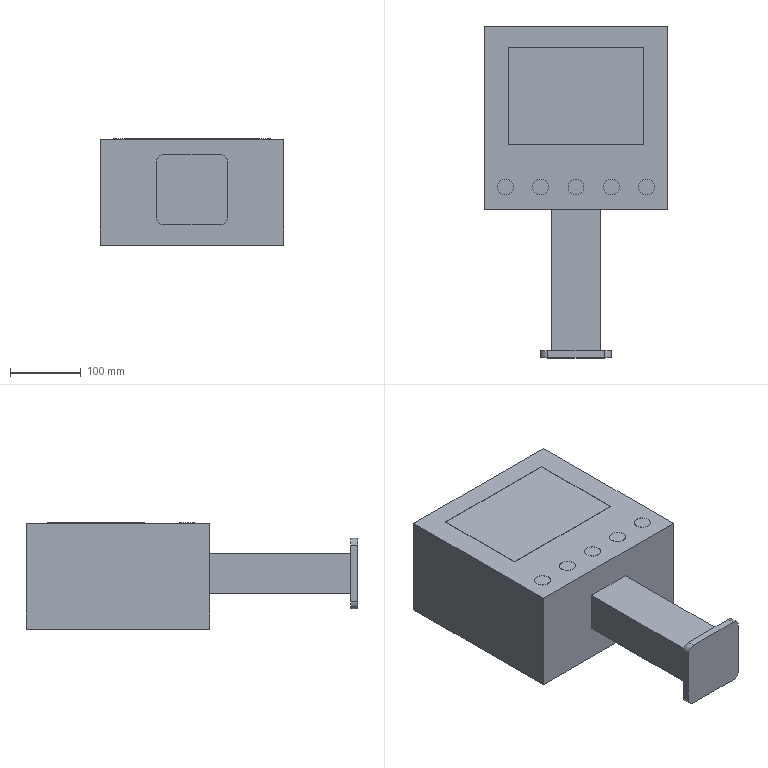Part | SolidWorks | features ICE 3, Extrusion 1, Fillet 1 | 1 solid | 40 faces | box 260 x 470 x 150.5 mm | volume 11032431 mm3 | plane 26 | cylinder 14 | commonest cylinder face diameters 22.5 x10 20 x4
STEP:
#1=CARTESIAN_POINT('',(11.25,-98.,150.5));
#2=VERTEX_POINT('',#1);
#3=CARTESIAN_POINT('',(-11.25,-98.,150.5));
#4=VERTEX_POINT('',#3);
#5=CARTESIAN_POINT('',(0.,-98.,150.5));
#6=DIRECTION('',(0.,0.,1.));
#7=DIRECTION('',(-1.,0.,0.));
#8=AXIS2_PLACEMENT_3D('',#5,#6,#7);
#9=CIRCLE('',#8,11.25);
#10=EDGE_CURVE('',#2,#4,#9,.T.);
#11=ORIENTED_EDGE('',*,*,#10,.F.);
#12=CARTESIAN_POINT('',(11.25,-98.,150.));
#13=VERTEX_POINT('',#12);
#14=CARTESIAN_POINT('',(11.25,-98.,150.5));
#15=DIRECTION('',(0.,0.,-1.));
#16=VECTOR('',#15,1000.);
#17=LINE('',#14,#16);
#18=EDGE_CURVE('',#2,#13,#17,.T.);
#19=ORIENTED_EDGE('',*,*,#18,.T.);
#20=CARTESIAN_POINT('',(-11.25,-98.,150.));
#21=VERTEX_POINT('',#20);
#22=CARTESIAN_POINT('',(0.,-98.,150.));
#23=DIRECTION('',(0.,0.,1.));
#24=DIRECTION('',(-1.,0.,0.));
#25=AXIS2_PLACEMENT_3D('',#22,#23,#24);
#26=CIRCLE('',#25,11.25);
#27=EDGE_CURVE('',#13,#21,#26,.T.);
#28=ORIENTED_EDGE('',*,*,#27,.T.);
#29=CARTESIAN_POINT('',(-11.25,-98.,150.5));
#30=DIRECTION('',(0.,0.,-1.));
#31=VECTOR('',#30,1000.);
#32=LINE('',#29,#31);
#33=EDGE_CURVE('',#4,#21,#32,.T.);
#34=ORIENTED_EDGE('',*,*,#33,.F.);
#35=EDGE_LOOP('',(#11,#19,#28,#34));
#36=FACE_OUTER_BOUND('',#35,.T.);
#37=CARTESIAN_POINT('',(0.,-98.,150.5));
#38=DIRECTION('',(0.,0.,-1.));
#39=DIRECTION('',(-1.,0.,0.));
#40=AXIS2_PLACEMENT_3D('',#37,#38,#39);
#41=CYLINDRICAL_SURFACE('',#40,11.25);
#42=ADVANCED_FACE('',(#36),#41,.T.);
#43=CARTESIAN_POINT('',(111.25,-98.,150.5));
#44=VERTEX_POINT('',#43);
#45=CARTESIAN_POINT('',(88.75,-98.,150.5));
#46=VERTEX_POINT('',#45);
#47=CARTESIAN_POINT('',(100.,-98.,150.5));
#48=DIRECTION('',(0.,0.,1.));
#49=DIRECTION('',(-1.,0.,0.));
#50=AXIS2_PLACEMENT_3D('',#47,#48,#49);
#51=CIRCLE('',#50,11.25);
#52=EDGE_CURVE('',#44,#46,#51,.T.);
#53=ORIENTED_EDGE('',*,*,#52,.F.);
#54=CARTESIAN_POINT('',(111.25,-98.,150.));
#55=VERTEX_POINT('',#54);
#56=CARTESIAN_POINT('',(111.25,-98.,150.5));
#57=DIRECTION('',(0.,0.,-1.));
#58=VECTOR('',#57,1000.);
#59=LINE('',#56,#58);
#60=EDGE_CURVE('',#44,#55,#59,.T.);
#61=ORIENTED_EDGE('',*,*,#60,.T.);
#62=CARTESIAN_POINT('',(88.75,-98.,150.));
#63=VERTEX_POINT('',#62);
#64=CARTESIAN_POINT('',(100.,-98.,150.));
#65=DIRECTION('',(0.,0.,1.));
#66=DIRECTION('',(-1.,0.,0.));
#67=AXIS2_PLACEMENT_3D('',#64,#65,#66);
#68=CIRCLE('',#67,11.25);
#69=EDGE_CURVE('',#55,#63,#68,.T.);
#70=ORIENTED_EDGE('',*,*,#69,.T.);
#71=CARTESIAN_POINT('',(88.75,-98.,150.5));
#72=DIRECTION('',(0.,0.,-1.));
#73=VECTOR('',#72,1000.);
#74=LINE('',#71,#73);
#75=EDGE_CURVE('',#46,#63,#74,.T.);
#76=ORIENTED_EDGE('',*,*,#75,.F.);
#77=EDGE_LOOP('',(#53,#61,#70,#76));
#78=FACE_OUTER_BOUND('',#77,.T.);
#79=CARTESIAN_POINT('',(100.,-98.,150.5));
#80=DIRECTION('',(0.,0.,-1.));
#81=DIRECTION('',(-1.,0.,0.));
#82=AXIS2_PLACEMENT_3D('',#79,#80,#81);
#83=CYLINDRICAL_SURFACE('',#82,11.25);
#84=ADVANCED_FACE('',(#78),#83,.T.);
#85=CARTESIAN_POINT('',(61.25,-98.,150.5));
#86=VERTEX_POINT('',#85);
#87=CARTESIAN_POINT('',(38.75,-98.,150.5));
#88=VERTEX_POINT('',#87);
#89=CARTESIAN_POINT('',(50.,-98.,150.5));
#90=DIRECTION('',(0.,0.,1.));
#91=DIRECTION('',(-1.,0.,0.));
#92=AXIS2_PLACEMENT_3D('',#89,#90,#91);
#93=CIRCLE('',#92,11.25);
#94=EDGE_CURVE('',#86,#88,#93,.T.);
#95=ORIENTED_EDGE('',*,*,#94,.F.);
#96=CARTESIAN_POINT('',(61.25,-98.,150.));
#97=VERTEX_POINT('',#96);
#98=CARTESIAN_POINT('',(61.25,-98.,150.5));
#99=DIRECTION('',(0.,0.,-1.));
#100=VECTOR('',#99,1000.);
#101=LINE('',#98,#100);
#102=EDGE_CURVE('',#86,#97,#101,.T.);
#103=ORIENTED_EDGE('',*,*,#102,.T.);
#104=CARTESIAN_POINT('',(38.75,-98.,150.));
#105=VERTEX_POINT('',#104);
#106=CARTESIAN_POINT('',(50.,-98.,150.));
#107=DIRECTION('',(0.,0.,1.));
#108=DIRECTION('',(-1.,0.,0.));
#109=AXIS2_PLACEMENT_3D('',#106,#107,#108);
#110=CIRCLE('',#109,11.25);
#111=EDGE_CURVE('',#97,#105,#110,.T.);
#112=ORIENTED_EDGE('',*,*,#111,.T.);
#113=CARTESIAN_POINT('',(38.75,-98.,150.5));
#114=DIRECTION('',(0.,0.,-1.));
#115=VECTOR('',#114,1000.);
#116=LINE('',#113,#115);
#117=EDGE_CURVE('',#88,#105,#116,.T.);
#118=ORIENTED_EDGE('',*,*,#117,.F.);
#119=EDGE_LOOP('',(#95,#103,#112,#118));
#120=FACE_OUTER_BOUND('',#119,.T.);
#121=CARTESIAN_POINT('',(50.,-98.,150.5));
#122=DIRECTION('',(0.,0.,-1.));
#123=DIRECTION('',(-1.,0.,0.));
#124=AXIS2_PLACEMENT_3D('',#121,#122,#123);
#125=CYLINDRICAL_SURFACE('',#124,11.25);
#126=ADVANCED_FACE('',(#120),#125,.T.);
#127=CARTESIAN_POINT('',(-38.75,-98.,150.5));
#128=VERTEX_POINT('',#127);
#129=CARTESIAN_POINT('',(-61.25,-98.,150.5));
#130=VERTEX_POINT('',#129);
#131=CARTESIAN_POINT('',(-50.,-98.,150.5));
#132=DIRECTION('',(0.,0.,1.));
#133=DIRECTION('',(1.,0.,0.));
#134=AXIS2_PLACEMENT_3D('',#131,#132,#133);
#135=CIRCLE('',#134,11.25);
#136=EDGE_CURVE('',#128,#130,#135,.T.);
#137=ORIENTED_EDGE('',*,*,#136,.F.);
#138=CARTESIAN_POINT('',(-38.75,-98.,150.));
#139=VERTEX_POINT('',#138);
#140=CARTESIAN_POINT('',(-38.75,-98.,150.5));
#141=DIRECTION('',(0.,0.,-1.));
#142=VECTOR('',#141,1000.);
#143=LINE('',#140,#142);
#144=EDGE_CURVE('',#128,#139,#143,.T.);
#145=ORIENTED_EDGE('',*,*,#144,.T.);
#146=CARTESIAN_POINT('',(-61.25,-98.,150.));
#147=VERTEX_POINT('',#146);
#148=CARTESIAN_POINT('',(-50.,-98.,150.));
#149=DIRECTION('',(0.,0.,1.));
#150=DIRECTION('',(1.,0.,0.));
#151=AXIS2_PLACEMENT_3D('',#148,#149,#150);
#152=CIRCLE('',#151,11.25);
#153=EDGE_CURVE('',#139,#147,#152,.T.);
#154=ORIENTED_EDGE('',*,*,#153,.T.);
#155=CARTESIAN_POINT('',(-61.25,-98.,150.5));
#156=DIRECTION('',(0.,0.,-1.));
#157=VECTOR('',#156,1000.);
#158=LINE('',#155,#157);
#159=EDGE_CURVE('',#130,#147,#158,.T.);
#160=ORIENTED_EDGE('',*,*,#159,.F.);
#161=EDGE_LOOP('',(#137,#145,#154,#160));
#162=FACE_OUTER_BOUND('',#161,.T.);
#163=CARTESIAN_POINT('',(-50.,-98.,150.5));
#164=DIRECTION('',(0.,0.,-1.));
#165=DIRECTION('',(-1.,0.,0.));
#166=AXIS2_PLACEMENT_3D('',#163,#164,#165);
#167=CYLINDRICAL_SURFACE('',#166,11.25);
#168=ADVANCED_FACE('',(#162),#167,.T.);
#169=CARTESIAN_POINT('',(-88.75,-98.,150.5));
#170=VERTEX_POINT('',#169);
#171=CARTESIAN_POINT('',(-111.25,-98.,150.5));
#172=VERTEX_POINT('',#171);
#173=CARTESIAN_POINT('',(-100.,-98.,150.5));
#174=DIRECTION('',(0.,0.,1.));
#175=DIRECTION('',(1.,0.,0.));
#176=AXIS2_PLACEMENT_3D('',#173,#174,#175);
#177=CIRCLE('',#176,11.25);
#178=EDGE_CURVE('',#170,#172,#177,.T.);
#179=ORIENTED_EDGE('',*,*,#178,.F.);
#180=CARTESIAN_POINT('',(-88.75,-98.,150.));
#181=VERTEX_POINT('',#180);
#182=CARTESIAN_POINT('',(-88.75,-98.,150.5));
#183=DIRECTION('',(0.,0.,-1.));
#184=VECTOR('',#183,1000.);
#185=LINE('',#182,#184);
#186=EDGE_CURVE('',#170,#181,#185,.T.);
#187=ORIENTED_EDGE('',*,*,#186,.T.);
#188=CARTESIAN_POINT('',(-111.25,-98.,150.));
#189=VERTEX_POINT('',#188);
#190=CARTESIAN_POINT('',(-100.,-98.,150.));
#191=DIRECTION('',(0.,0.,1.));
#192=DIRECTION('',(1.,0.,0.));
#193=AXIS2_PLACEMENT_3D('',#190,#191,#192);
#194=CIRCLE('',#193,11.25);
#195=EDGE_CURVE('',#181,#189,#194,.T.);
#196=ORIENTED_EDGE('',*,*,#195,.T.);
#197=CARTESIAN_POINT('',(-111.25,-98.,150.5));
#198=DIRECTION('',(0.,0.,-1.));
#199=VECTOR('',#198,1000.);
#200=LINE('',#197,#199);
#201=EDGE_CURVE('',#172,#189,#200,.T.);
#202=ORIENTED_EDGE('',*,*,#201,.F.);
#203=EDGE_LOOP('',(#179,#187,#196,#202));
#204=FACE_OUTER_BOUND('',#203,.T.);
#205=CARTESIAN_POINT('',(-100.,-98.,150.5));
#206=DIRECTION('',(0.,0.,-1.));
#207=DIRECTION('',(-1.,0.,0.));
#208=AXIS2_PLACEMENT_3D('',#205,#206,#207);
#209=CYLINDRICAL_SURFACE('',#208,11.25);
#210=ADVANCED_FACE('',(#204),#209,.T.);
#211=CARTESIAN_POINT('',(-130.,-130.,0.));
#212=VERTEX_POINT('',#211);
#213=CARTESIAN_POINT('',(130.,-130.,0.));
#214=VERTEX_POINT('',#213);
#215=CARTESIAN_POINT('',(-130.,-130.,0.));
#216=DIRECTION('',(1.,0.,0.));
#217=VECTOR('',#216,1000.);
#218=LINE('',#215,#217);
#219=EDGE_CURVE('',#212,#214,#218,.T.);
#220=ORIENTED_EDGE('',*,*,#219,.T.);
#221=CARTESIAN_POINT('',(130.,-130.,150.));
#222=VERTEX_POINT('',#221);
#223=CARTESIAN_POINT('',(130.,-130.,150.));
#224=DIRECTION('',(0.,0.,-1.));
#225=VECTOR('',#224,1000.);
#226=LINE('',#223,#225);
#227=EDGE_CURVE('',#222,#214,#226,.T.);
#228=ORIENTED_EDGE('',*,*,#227,.F.);
#229=CARTESIAN_POINT('',(-130.,-130.,150.));
#230=VERTEX_POINT('',#229);
#231=CARTESIAN_POINT('',(-130.,-130.,150.));
#232=DIRECTION('',(1.,0.,0.));
#233=VECTOR('',#232,1000.);
#234=LINE('',#231,#233);
#235=EDGE_CURVE('',#230,#222,#234,.T.);
#236=ORIENTED_EDGE('',*,*,#235,.F.);
#237=CARTESIAN_POINT('',(-130.,-130.,150.));
#238=DIRECTION('',(0.,0.,-1.));
#239=VECTOR('',#238,1000.);
#240=LINE('',#237,#239);
#241=EDGE_CURVE('',#230,#212,#240,.T.);
#242=ORIENTED_EDGE('',*,*,#241,.T.);
#243=EDGE_LOOP('',(#220,#228,#236,#242));
#244=FACE_OUTER_BOUND('',#243,.T.);
#245=CARTESIAN_POINT('',(34.037,-130.,49.969));
#246=VERTEX_POINT('',#245);
#247=CARTESIAN_POINT('',(34.037,-130.,107.19));
#248=VERTEX_POINT('',#247);
#249=CARTESIAN_POINT('',(34.037,-130.,107.19));
#250=DIRECTION('',(0.,0.,1.));
#251=VECTOR('',#250,1000.);
#252=LINE('',#249,#251);
#253=EDGE_CURVE('',#246,#248,#252,.T.);
#254=ORIENTED_EDGE('',*,*,#253,.F.);
#255=CARTESIAN_POINT('',(-34.037,-130.,49.969));
#256=VERTEX_POINT('',#255);
#257=CARTESIAN_POINT('',(-34.037,-130.,49.969));
#258=DIRECTION('',(1.,0.,0.));
#259=VECTOR('',#258,1000.);
#260=LINE('',#257,#259);
#261=EDGE_CURVE('',#256,#246,#260,.T.);
#262=ORIENTED_EDGE('',*,*,#261,.F.);
#263=CARTESIAN_POINT('',(-34.037,-130.,107.19));
#264=VERTEX_POINT('',#263);
#265=CARTESIAN_POINT('',(-34.037,-130.,107.19));
#266=DIRECTION('',(0.,0.,-1.));
#267=VECTOR('',#266,1000.);
#268=LINE('',#265,#267);
#269=EDGE_CURVE('',#264,#256,#268,.T.);
#270=ORIENTED_EDGE('',*,*,#269,.F.);
#271=CARTESIAN_POINT('',(-34.037,-130.,107.19));
#272=DIRECTION('',(-1.,0.,0.));
#273=VECTOR('',#272,1000.);
#274=LINE('',#271,#273);
#275=EDGE_CURVE('',#248,#264,#274,.T.);
#276=ORIENTED_EDGE('',*,*,#275,.F.);
#277=EDGE_LOOP('',(#254,#262,#270,#276));
#278=FACE_BOUND('',#277,.T.);
#279=CARTESIAN_POINT('',(-130.,-130.,150.));
#280=DIRECTION('',(0.,1.,0.));
#281=DIRECTION('',(0.,0.,1.));
#282=AXIS2_PLACEMENT_3D('',#279,#280,#281);
#283=PLANE('',#282);
#284=ADVANCED_FACE('',(#244,#278),#283,.F.);
#285=CARTESIAN_POINT('',(130.,130.,0.));
#286=VERTEX_POINT('',#285);
#287=CARTESIAN_POINT('',(130.,130.,0.));
#288=DIRECTION('',(0.,1.,0.));
#289=VECTOR('',#288,1000.);
#290=LINE('',#287,#289);
#291=EDGE_CURVE('',#214,#286,#290,.T.);
#292=ORIENTED_EDGE('',*,*,#291,.T.);
#293=CARTESIAN_POINT('',(130.,130.,150.));
#294=VERTEX_POINT('',#293);
#295=CARTESIAN_POINT('',(130.,130.,150.));
#296=DIRECTION('',(0.,0.,-1.));
#297=VECTOR('',#296,1000.);
#298=LINE('',#295,#297);
#299=EDGE_CURVE('',#294,#286,#298,.T.);
#300=ORIENTED_EDGE('',*,*,#299,.F.);
#301=CARTESIAN_POINT('',(130.,130.,150.));
#302=DIRECTION('',(0.,1.,0.));
#303=VECTOR('',#302,1000.);
#304=LINE('',#301,#303);
#305=EDGE_CURVE('',#222,#294,#304,.T.);
#306=ORIENTED_EDGE('',*,*,#305,.F.);
#307=ORIENTED_EDGE('',*,*,#227,.T.);
#308=EDGE_LOOP('',(#292,#300,#306,#307));
#309=FACE_OUTER_BOUND('',#308,.T.);
#310=CARTESIAN_POINT('',(130.,130.,150.));
#311=DIRECTION('',(-1.,0.,0.));
#312=DIRECTION('',(0.,-1.,0.));
#313=AXIS2_PLACEMENT_3D('',#310,#311,#312);
#314=PLANE('',#313);
#315=ADVANCED_FACE('',(#309),#314,.F.);
#316=CARTESIAN_POINT('',(-130.,130.,0.));
#317=VERTEX_POINT('',#316);
#318=CARTESIAN_POINT('',(-130.,130.,0.));
#319=DIRECTION('',(-1.,0.,0.));
#320=VECTOR('',#319,1000.);
#321=LINE('',#318,#320);
#322=EDGE_CURVE('',#286,#317,#321,.T.);
#323=ORIENTED_EDGE('',*,*,#322,.T.);
#324=CARTESIAN_POINT('',(-130.,130.,150.));
#325=VERTEX_POINT('',#324);
#326=CARTESIAN_POINT('',(-130.,130.,150.));
#327=DIRECTION('',(0.,0.,-1.));
#328=VECTOR('',#327,1000.);
#329=LINE('',#326,#328);
#330=EDGE_CURVE('',#325,#317,#329,.T.);
#331=ORIENTED_EDGE('',*,*,#330,.F.);
#332=CARTESIAN_POINT('',(-130.,130.,150.));
#333=DIRECTION('',(-1.,0.,0.));
#334=VECTOR('',#333,1000.);
#335=LINE('',#332,#334);
#336=EDGE_CURVE('',#294,#325,#335,.T.);
#337=ORIENTED_EDGE('',*,*,#336,.F.);
#338=ORIENTED_EDGE('',*,*,#299,.T.);
#339=EDGE_LOOP('',(#323,#331,#337,#338));
#340=FACE_OUTER_BOUND('',#339,.T.);
#341=CARTESIAN_POINT('',(-130.,130.,150.));
#342=DIRECTION('',(0.,-1.,0.));
#343=DIRECTION('',(0.,0.,-1.));
#344=AXIS2_PLACEMENT_3D('',#341,#342,#343);
#345=PLANE('',#344);
#346=ADVANCED_FACE('',(#340),#345,.F.);
#347=CARTESIAN_POINT('',(-130.,130.,0.));
#348=DIRECTION('',(0.,-1.,0.));
#349=VECTOR('',#348,1000.);
#350=LINE('',#347,#349);
#351=EDGE_CURVE('',#317,#212,#350,.T.);
#352=ORIENTED_EDGE('',*,*,#351,.T.);
#353=ORIENTED_EDGE('',*,*,#241,.F.);
#354=CARTESIAN_POINT('',(-130.,130.,150.));
#355=DIRECTION('',(0.,-1.,0.));
#356=VECTOR('',#355,1000.);
#357=LINE('',#354,#356);
#358=EDGE_CURVE('',#325,#230,#357,.T.);
#359=ORIENTED_EDGE('',*,*,#358,.F.);
#360=ORIENTED_EDGE('',*,*,#330,.T.);
#361=EDGE_LOOP('',(#352,#353,#359,#360));
#362=FACE_OUTER_BOUND('',#361,.T.);
#363=CARTESIAN_POINT('',(-130.,130.,150.));
#364=DIRECTION('',(1.,0.,0.));
#365=DIRECTION('',(0.,0.,-1.));
#366=AXIS2_PLACEMENT_3D('',#363,#364,#365);
#367=PLANE('',#366);
#368=ADVANCED_FACE('',(#362),#367,.F.);
#369=CARTESIAN_POINT('',(0.,-98.,150.));
#370=DIRECTION('',(0.,0.,1.));
#371=DIRECTION('',(-1.,0.,0.));
#372=AXIS2_PLACEMENT_3D('',#369,#370,#371);
#373=CIRCLE('',#372,11.25);
#374=EDGE_CURVE('',#21,#13,#373,.T.);
#375=ORIENTED_EDGE('',*,*,#374,.F.);
#376=ORIENTED_EDGE('',*,*,#27,.F.);
#377=EDGE_LOOP('',(#375,#376));
#378=FACE_BOUND('',#377,.T.);
#379=CARTESIAN_POINT('',(100.,-98.,150.));
#380=DIRECTION('',(0.,0.,1.));
#381=DIRECTION('',(-1.,0.,0.));
#382=AXIS2_PLACEMENT_3D('',#379,#380,#381);
#383=CIRCLE('',#382,11.25);
#384=EDGE_CURVE('',#63,#55,#383,.T.);
#385=ORIENTED_EDGE('',*,*,#384,.F.);
#386=ORIENTED_EDGE('',*,*,#69,.F.);
#387=EDGE_LOOP('',(#385,#386));
#388=FACE_BOUND('',#387,.T.);
#389=CARTESIAN_POINT('',(50.,-98.,150.));
#390=DIRECTION('',(0.,0.,1.));
#391=DIRECTION('',(-1.,0.,0.));
#392=AXIS2_PLACEMENT_3D('',#389,#390,#391);
#393=CIRCLE('',#392,11.25);
#394=EDGE_CURVE('',#105,#97,#393,.T.);
#395=ORIENTED_EDGE('',*,*,#394,.F.);
#396=ORIENTED_EDGE('',*,*,#111,.F.);
#397=EDGE_LOOP('',(#395,#396));
#398=FACE_BOUND('',#397,.T.);
#399=CARTESIAN_POINT('',(-50.,-98.,150.));
#400=DIRECTION('',(0.,0.,1.));
#401=DIRECTION('',(1.,0.,0.));
#402=AXIS2_PLACEMENT_3D('',#399,#400,#401);
#403=CIRCLE('',#402,11.25);
#404=EDGE_CURVE('',#147,#139,#403,.T.);
#405=ORIENTED_EDGE('',*,*,#404,.F.);
#406=ORIENTED_EDGE('',*,*,#153,.F.);
#407=EDGE_LOOP('',(#405,#406));
#408=FACE_BOUND('',#407,.T.);
#409=CARTESIAN_POINT('',(-100.,-98.,150.));
#410=DIRECTION('',(0.,0.,1.));
#411=DIRECTION('',(1.,0.,0.));
#412=AXIS2_PLACEMENT_3D('',#409,#410,#411);
#413=CIRCLE('',#412,11.25);
#414=EDGE_CURVE('',#189,#181,#413,.T.);
#415=ORIENTED_EDGE('',*,*,#414,.F.);
#416=ORIENTED_EDGE('',*,*,#195,.F.);
#417=EDGE_LOOP('',(#415,#416));
#418=FACE_BOUND('',#417,.T.);
#419=CARTESIAN_POINT('',(-96.,100.,150.));
#420=VERTEX_POINT('',#419);
#421=CARTESIAN_POINT('',(-96.,-38.,150.));
#422=VERTEX_POINT('',#421);
#423=CARTESIAN_POINT('',(-96.,100.,150.));
#424=DIRECTION('',(0.,-1.,0.));
#425=VECTOR('',#424,1000.);
#426=LINE('',#423,#425);
#427=EDGE_CURVE('',#420,#422,#426,.T.);
#428=ORIENTED_EDGE('',*,*,#427,.F.);
#429=CARTESIAN_POINT('',(96.,100.,150.));
#430=VERTEX_POINT('',#429);
#431=CARTESIAN_POINT('',(-96.,100.,150.));
#432=DIRECTION('',(-1.,0.,0.));
#433=VECTOR('',#432,1000.);
#434=LINE('',#431,#433);
#435=EDGE_CURVE('',#430,#420,#434,.T.);
#436=ORIENTED_EDGE('',*,*,#435,.F.);
#437=CARTESIAN_POINT('',(96.,-38.,150.));
#438=VERTEX_POINT('',#437);
#439=CARTESIAN_POINT('',(96.,100.,150.));
#440=DIRECTION('',(0.,1.,0.));
#441=VECTOR('',#440,1000.);
#442=LINE('',#439,#441);
#443=EDGE_CURVE('',#438,#430,#442,.T.);
#444=ORIENTED_EDGE('',*,*,#443,.F.);
#445=CARTESIAN_POINT('',(-96.,-38.,150.));
#446=DIRECTION('',(1.,0.,0.));
#447=VECTOR('',#446,1000.);
#448=LINE('',#445,#447);
#449=EDGE_CURVE('',#422,#438,#448,.T.);
#450=ORIENTED_EDGE('',*,*,#449,.F.);
#451=EDGE_LOOP('',(#428,#436,#444,#450));
#452=FACE_BOUND('',#451,.T.);
#453=ORIENTED_EDGE('',*,*,#305,.T.);
#454=ORIENTED_EDGE('',*,*,#336,.T.);
#455=ORIENTED_EDGE('',*,*,#358,.T.);
#456=ORIENTED_EDGE('',*,*,#235,.T.);
#457=EDGE_LOOP('',(#453,#454,#455,#456));
#458=FACE_OUTER_BOUND('',#457,.T.);
#459=CARTESIAN_POINT('',(0.,0.,150.));
#460=DIRECTION('',(0.,0.,1.));
#461=DIRECTION('',(1.,0.,0.));
#462=AXIS2_PLACEMENT_3D('',#459,#460,#461);
#463=PLANE('',#462);
#464=ADVANCED_FACE('',(#378,#388,#398,#408,#418,#452,#458),#463,.T.);
#465=ORIENTED_EDGE('',*,*,#291,.F.);
#466=ORIENTED_EDGE('',*,*,#219,.F.);
#467=ORIENTED_EDGE('',*,*,#351,.F.);
#468=ORIENTED_EDGE('',*,*,#322,.F.);
#469=EDGE_LOOP('',(#465,#466,#467,#468));
#470=FACE_OUTER_BOUND('',#469,.T.);
#471=CARTESIAN_POINT('',(0.,0.,0.));
#472=DIRECTION('',(0.,0.,1.));
#473=DIRECTION('',(1.,0.,0.));
#474=AXIS2_PLACEMENT_3D('',#471,#472,#473);
#475=PLANE('',#474);
#476=ADVANCED_FACE('',(#470),#475,.F.);
#477=ORIENTED_EDGE('',*,*,#427,.T.);
#478=CARTESIAN_POINT('',(-96.,-38.,150.5));
#479=VERTEX_POINT('',#478);
#480=CARTESIAN_POINT('',(-96.,-38.,150.5));
#481=DIRECTION('',(0.,0.,-1.));
#482=VECTOR('',#481,1000.);
#483=LINE('',#480,#482);
#484=EDGE_CURVE('',#479,#422,#483,.T.);
#485=ORIENTED_EDGE('',*,*,#484,.F.);
#486=CARTESIAN_POINT('',(-96.,100.,150.5));
#487=VERTEX_POINT('',#486);
#488=CARTESIAN_POINT('',(-96.,100.,150.5));
#489=DIRECTION('',(0.,-1.,0.));
#490=VECTOR('',#489,1000.);
#491=LINE('',#488,#490);
#492=EDGE_CURVE('',#487,#479,#491,.T.);
#493=ORIENTED_EDGE('',*,*,#492,.F.);
#494=CARTESIAN_POINT('',(-96.,100.,150.5));
#495=DIRECTION('',(0.,0.,-1.));
#496=VECTOR('',#495,1000.);
#497=LINE('',#494,#496);
#498=EDGE_CURVE('',#487,#420,#497,.T.);
#499=ORIENTED_EDGE('',*,*,#498,.T.);
#500=EDGE_LOOP('',(#477,#485,#493,#499));
#501=FACE_OUTER_BOUND('',#500,.T.);
#502=CARTESIAN_POINT('',(-96.,100.,150.5));
#503=DIRECTION('',(1.,0.,0.));
#504=DIRECTION('',(0.,0.,-1.));
#505=AXIS2_PLACEMENT_3D('',#502,#503,#504);
#506=PLANE('',#505);
#507=ADVANCED_FACE('',(#501),#506,.F.);
#508=ORIENTED_EDGE('',*,*,#449,.T.);
#509=CARTESIAN_POINT('',(96.,-38.,150.5));
#510=VERTEX_POINT('',#509);
#511=CARTESIAN_POINT('',(96.,-38.,150.5));
#512=DIRECTION('',(0.,0.,-1.));
#513=VECTOR('',#512,1000.);
#514=LINE('',#511,#513);
#515=EDGE_CURVE('',#510,#438,#514,.T.);
#516=ORIENTED_EDGE('',*,*,#515,.F.);
#517=CARTESIAN_POINT('',(-96.,-38.,150.5));
#518=DIRECTION('',(1.,0.,0.));
#519=VECTOR('',#518,1000.);
#520=LINE('',#517,#519);
#521=EDGE_CURVE('',#479,#510,#520,.T.);
#522=ORIENTED_EDGE('',*,*,#521,.F.);
#523=ORIENTED_EDGE('',*,*,#484,.T.);
#524=EDGE_LOOP('',(#508,#516,#522,#523));
#525=FACE_OUTER_BOUND('',#524,.T.);
#526=CARTESIAN_POINT('',(-96.,-38.,150.5));
#527=DIRECTION('',(0.,1.,0.));
#528=DIRECTION('',(-1.,0.,0.));
#529=AXIS2_PLACEMENT_3D('',#526,#527,#528);
#530=PLANE('',#529);
#531=ADVANCED_FACE('',(#525),#530,.F.);
#532=ORIENTED_EDGE('',*,*,#443,.T.);
#533=CARTESIAN_POINT('',(96.,100.,150.5));
#534=VERTEX_POINT('',#533);
#535=CARTESIAN_POINT('',(96.,100.,150.5));
#536=DIRECTION('',(0.,0.,-1.));
#537=VECTOR('',#536,1000.);
#538=LINE('',#535,#537);
#539=EDGE_CURVE('',#534,#430,#538,.T.);
#540=ORIENTED_EDGE('',*,*,#539,.F.);
#541=CARTESIAN_POINT('',(96.,100.,150.5));
#542=DIRECTION('',(0.,1.,0.));
#543=VECTOR('',#542,1000.);
#544=LINE('',#541,#543);
#545=EDGE_CURVE('',#510,#534,#544,.T.);
#546=ORIENTED_EDGE('',*,*,#545,.F.);
#547=ORIENTED_EDGE('',*,*,#515,.T.);
#548=EDGE_LOOP('',(#532,#540,#546,#547));
#549=FACE_OUTER_BOUND('',#548,.T.);
#550=CARTESIAN_POINT('',(96.,100.,150.5));
#551=DIRECTION('',(-1.,0.,0.));
#552=DIRECTION('',(0.,-1.,0.));
#553=AXIS2_PLACEMENT_3D('',#550,#551,#552);
#554=PLANE('',#553);
#555=ADVANCED_FACE('',(#549),#554,.F.);
#556=ORIENTED_EDGE('',*,*,#435,.T.);
#557=ORIENTED_EDGE('',*,*,#498,.F.);
#558=CARTESIAN_POINT('',(-96.,100.,150.5));
#559=DIRECTION('',(-1.,0.,0.));
#560=VECTOR('',#559,1000.);
#561=LINE('',#558,#560);
#562=EDGE_CURVE('',#534,#487,#561,.T.);
#563=ORIENTED_EDGE('',*,*,#562,.F.);
#564=ORIENTED_EDGE('',*,*,#539,.T.);
#565=EDGE_LOOP('',(#556,#557,#563,#564));
#566=FACE_OUTER_BOUND('',#565,.T.);
#567=CARTESIAN_POINT('',(-96.,100.,150.5));
#568=DIRECTION('',(0.,-1.,0.));
#569=DIRECTION('',(1.,0.,0.));
#570=AXIS2_PLACEMENT_3D('',#567,#568,#569);
#571=PLANE('',#570);
#572=ADVANCED_FACE('',(#566),#571,.F.);
#573=ORIENTED_EDGE('',*,*,#492,.T.);
#574=ORIENTED_EDGE('',*,*,#521,.T.);
#575=ORIENTED_EDGE('',*,*,#545,.T.);
#576=ORIENTED_EDGE('',*,*,#562,.T.);
#577=EDGE_LOOP('',(#573,#574,#575,#576));
#578=FACE_OUTER_BOUND('',#577,.T.);
#579=CARTESIAN_POINT('',(0.,0.,150.5));
#580=DIRECTION('',(0.,0.,1.));
#581=DIRECTION('',(1.,0.,0.));
#582=AXIS2_PLACEMENT_3D('',#579,#580,#581);
#583=PLANE('',#582);
#584=ADVANCED_FACE('',(#578),#583,.T.);
#585=ORIENTED_EDGE('',*,*,#186,.F.);
#586=CARTESIAN_POINT('',(-100.,-98.,150.5));
#587=DIRECTION('',(0.,0.,1.));
#588=DIRECTION('',(1.,0.,0.));
#589=AXIS2_PLACEMENT_3D('',#586,#587,#588);
#590=CIRCLE('',#589,11.25);
#591=EDGE_CURVE('',#172,#170,#590,.T.);
#592=ORIENTED_EDGE('',*,*,#591,.F.);
#593=ORIENTED_EDGE('',*,*,#201,.T.);
#594=ORIENTED_EDGE('',*,*,#414,.T.);
#595=EDGE_LOOP('',(#585,#592,#593,#594));
#596=FACE_OUTER_BOUND('',#595,.T.);
#597=CARTESIAN_POINT('',(-100.,-98.,150.5));
#598=DIRECTION('',(0.,0.,-1.));
#599=DIRECTION('',(-1.,0.,0.));
#600=AXIS2_PLACEMENT_3D('',#597,#598,#599);
#601=CYLINDRICAL_SURFACE('',#600,11.25);
#602=ADVANCED_FACE('',(#596),#601,.T.);
#603=ORIENTED_EDGE('',*,*,#591,.T.);
#604=ORIENTED_EDGE('',*,*,#178,.T.);
#605=EDGE_LOOP('',(#603,#604));
#606=FACE_OUTER_BOUND('',#605,.T.);
#607=CARTESIAN_POINT('',(-100.,-98.,150.5));
#608=DIRECTION('',(0.,0.,1.));
#609=DIRECTION('',(1.,0.,0.));
#610=AXIS2_PLACEMENT_3D('',#607,#608,#609);
#611=PLANE('',#610);
#612=ADVANCED_FACE('',(#606),#611,.T.);
#613=ORIENTED_EDGE('',*,*,#144,.F.);
#614=CARTESIAN_POINT('',(-50.,-98.,150.5));
#615=DIRECTION('',(0.,0.,1.));
#616=DIRECTION('',(1.,0.,0.));
#617=AXIS2_PLACEMENT_3D('',#614,#615,#616);
#618=CIRCLE('',#617,11.25);
#619=EDGE_CURVE('',#130,#128,#618,.T.);
#620=ORIENTED_EDGE('',*,*,#619,.F.);
#621=ORIENTED_EDGE('',*,*,#159,.T.);
#622=ORIENTED_EDGE('',*,*,#404,.T.);
#623=EDGE_LOOP('',(#613,#620,#621,#622));
#624=FACE_OUTER_BOUND('',#623,.T.);
#625=CARTESIAN_POINT('',(-50.,-98.,150.5));
#626=DIRECTION('',(0.,0.,-1.));
#627=DIRECTION('',(-1.,0.,0.));
#628=AXIS2_PLACEMENT_3D('',#625,#626,#627);
#629=CYLINDRICAL_SURFACE('',#628,11.25);
#630=ADVANCED_FACE('',(#624),#629,.T.);
#631=ORIENTED_EDGE('',*,*,#619,.T.);
#632=ORIENTED_EDGE('',*,*,#136,.T.);
#633=EDGE_LOOP('',(#631,#632));
#634=FACE_OUTER_BOUND('',#633,.T.);
#635=CARTESIAN_POINT('',(-50.,-98.,150.5));
#636=DIRECTION('',(0.,0.,1.));
#637=DIRECTION('',(1.,0.,0.));
#638=AXIS2_PLACEMENT_3D('',#635,#636,#637);
#639=PLANE('',#638);
#640=ADVANCED_FACE('',(#634),#639,.T.);
#641=ORIENTED_EDGE('',*,*,#102,.F.);
#642=CARTESIAN_POINT('',(50.,-98.,150.5));
#643=DIRECTION('',(0.,0.,1.));
#644=DIRECTION('',(-1.,0.,0.));
#645=AXIS2_PLACEMENT_3D('',#642,#643,#644);
#646=CIRCLE('',#645,11.25);
#647=EDGE_CURVE('',#88,#86,#646,.T.);
#648=ORIENTED_EDGE('',*,*,#647,.F.);
#649=ORIENTED_EDGE('',*,*,#117,.T.);
#650=ORIENTED_EDGE('',*,*,#394,.T.);
#651=EDGE_LOOP('',(#641,#648,#649,#650));
#652=FACE_OUTER_BOUND('',#651,.T.);
#653=CARTESIAN_POINT('',(50.,-98.,150.5));
#654=DIRECTION('',(0.,0.,-1.));
#655=DIRECTION('',(-1.,0.,0.));
#656=AXIS2_PLACEMENT_3D('',#653,#654,#655);
#657=CYLINDRICAL_SURFACE('',#656,11.25);
#658=ADVANCED_FACE('',(#652),#657,.T.);
#659=ORIENTED_EDGE('',*,*,#647,.T.);
#660=ORIENTED_EDGE('',*,*,#94,.T.);
#661=EDGE_LOOP('',(#659,#660));
#662=FACE_OUTER_BOUND('',#661,.T.);
#663=CARTESIAN_POINT('',(50.,-98.,150.5));
#664=DIRECTION('',(0.,0.,-1.));
#665=DIRECTION('',(-1.,0.,0.));
#666=AXIS2_PLACEMENT_3D('',#663,#664,#665);
#667=PLANE('',#666);
#668=ADVANCED_FACE('',(#662),#667,.F.);
#669=ORIENTED_EDGE('',*,*,#60,.F.);
#670=CARTESIAN_POINT('',(100.,-98.,150.5));
#671=DIRECTION('',(0.,0.,1.));
#672=DIRECTION('',(-1.,0.,0.));
#673=AXIS2_PLACEMENT_3D('',#670,#671,#672);
#674=CIRCLE('',#673,11.25);
#675=EDGE_CURVE('',#46,#44,#674,.T.);
#676=ORIENTED_EDGE('',*,*,#675,.F.);
#677=ORIENTED_EDGE('',*,*,#75,.T.);
#678=ORIENTED_EDGE('',*,*,#384,.T.);
#679=EDGE_LOOP('',(#669,#676,#677,#678));
#680=FACE_OUTER_BOUND('',#679,.T.);
#681=CARTESIAN_POINT('',(100.,-98.,150.5));
#682=DIRECTION('',(0.,0.,-1.));
#683=DIRECTION('',(-1.,0.,0.));
#684=AXIS2_PLACEMENT_3D('',#681,#682,#683);
#685=CYLINDRICAL_SURFACE('',#684,11.25);
#686=ADVANCED_FACE('',(#680),#685,.T.);
#687=ORIENTED_EDGE('',*,*,#675,.T.);
#688=ORIENTED_EDGE('',*,*,#52,.T.);
#689=EDGE_LOOP('',(#687,#688));
#690=FACE_OUTER_BOUND('',#689,.T.);
#691=CARTESIAN_POINT('',(100.,-98.,150.5));
#692=DIRECTION('',(0.,0.,-1.));
#693=DIRECTION('',(-1.,0.,0.));
#694=AXIS2_PLACEMENT_3D('',#691,#692,#693);
#695=PLANE('',#694);
#696=ADVANCED_FACE('',(#690),#695,.F.);
#697=ORIENTED_EDGE('',*,*,#18,.F.);
#698=CARTESIAN_POINT('',(0.,-98.,150.5));
#699=DIRECTION('',(0.,0.,1.));
#700=DIRECTION('',(-1.,0.,0.));
#701=AXIS2_PLACEMENT_3D('',#698,#699,#700);
#702=CIRCLE('',#701,11.25);
#703=EDGE_CURVE('',#4,#2,#702,.T.);
#704=ORIENTED_EDGE('',*,*,#703,.F.);
#705=ORIENTED_EDGE('',*,*,#33,.T.);
#706=ORIENTED_EDGE('',*,*,#374,.T.);
#707=EDGE_LOOP('',(#697,#704,#705,#706));
#708=FACE_OUTER_BOUND('',#707,.T.);
#709=CARTESIAN_POINT('',(0.,-98.,150.5));
#710=DIRECTION('',(0.,0.,-1.));
#711=DIRECTION('',(-1.,0.,0.));
#712=AXIS2_PLACEMENT_3D('',#709,#710,#711);
#713=CYLINDRICAL_SURFACE('',#712,11.25);
#714=ADVANCED_FACE('',(#708),#713,.T.);
#715=ORIENTED_EDGE('',*,*,#703,.T.);
#716=ORIENTED_EDGE('',*,*,#10,.T.);
#717=EDGE_LOOP('',(#715,#716));
#718=FACE_OUTER_BOUND('',#717,.T.);
#719=CARTESIAN_POINT('',(0.,-98.,150.5));
#720=DIRECTION('',(0.,0.,-1.));
#721=DIRECTION('',(-1.,0.,0.));
#722=AXIS2_PLACEMENT_3D('',#719,#720,#721);
#723=PLANE('',#722);
#724=ADVANCED_FACE('',(#718),#723,.F.);
#725=ORIENTED_EDGE('',*,*,#253,.T.);
#726=CARTESIAN_POINT('',(34.037,-330.,107.19));
#727=VERTEX_POINT('',#726);
#728=CARTESIAN_POINT('',(34.037,-330.,107.19));
#729=DIRECTION('',(0.,1.,0.));
#730=VECTOR('',#729,1000.);
#731=LINE('',#728,#730);
#732=EDGE_CURVE('',#727,#248,#731,.T.);
#733=ORIENTED_EDGE('',*,*,#732,.F.);
#734=CARTESIAN_POINT('',(34.037,-330.,49.969));
#735=VERTEX_POINT('',#734);
#736=CARTESIAN_POINT('',(34.037,-330.,107.19));
#737=DIRECTION('',(0.,0.,1.));
#738=VECTOR('',#737,1000.);
#739=LINE('',#736,#738);
#740=EDGE_CURVE('',#735,#727,#739,.T.);
#741=ORIENTED_EDGE('',*,*,#740,.F.);
#742=CARTESIAN_POINT('',(34.037,-330.,49.969));
#743=DIRECTION('',(0.,1.,0.));
#744=VECTOR('',#743,1000.);
#745=LINE('',#742,#744);
#746=EDGE_CURVE('',#735,#246,#745,.T.);
#747=ORIENTED_EDGE('',*,*,#746,.T.);
#748=EDGE_LOOP('',(#725,#733,#741,#747));
#749=FACE_OUTER_BOUND('',#748,.T.);
#750=CARTESIAN_POINT('',(34.037,-330.,107.19));
#751=DIRECTION('',(-1.,0.,0.));
#752=DIRECTION('',(0.,0.,1.));
#753=AXIS2_PLACEMENT_3D('',#750,#751,#752);
#754=PLANE('',#753);
#755=ADVANCED_FACE('',(#749),#754,.F.);
#756=ORIENTED_EDGE('',*,*,#275,.T.);
#757=CARTESIAN_POINT('',(-34.037,-330.,107.19));
#758=VERTEX_POINT('',#757);
#759=CARTESIAN_POINT('',(-34.037,-330.,107.19));
#760=DIRECTION('',(0.,1.,0.));
#761=VECTOR('',#760,1000.);
#762=LINE('',#759,#761);
#763=EDGE_CURVE('',#758,#264,#762,.T.);
#764=ORIENTED_EDGE('',*,*,#763,.F.);
#765=CARTESIAN_POINT('',(-34.037,-330.,107.19));
#766=DIRECTION('',(-1.,0.,0.));
#767=VECTOR('',#766,1000.);
#768=LINE('',#765,#767);
#769=EDGE_CURVE('',#727,#758,#768,.T.);
#770=ORIENTED_EDGE('',*,*,#769,.F.);
#771=ORIENTED_EDGE('',*,*,#732,.T.);
#772=EDGE_LOOP('',(#756,#764,#770,#771));
#773=FACE_OUTER_BOUND('',#772,.T.);
#774=CARTESIAN_POINT('',(-34.037,-330.,107.19));
#775=DIRECTION('',(0.,0.,-1.));
#776=DIRECTION('',(-1.,0.,0.));
#777=AXIS2_PLACEMENT_3D('',#774,#775,#776);
#778=PLANE('',#777);
#779=ADVANCED_FACE('',(#773),#778,.F.);
#780=ORIENTED_EDGE('',*,*,#269,.T.);
#781=CARTESIAN_POINT('',(-34.037,-330.,49.969));
#782=VERTEX_POINT('',#781);
#783=CARTESIAN_POINT('',(-34.037,-330.,49.969));
#784=DIRECTION('',(0.,1.,0.));
#785=VECTOR('',#784,1000.);
#786=LINE('',#783,#785);
#787=EDGE_CURVE('',#782,#256,#786,.T.);
#788=ORIENTED_EDGE('',*,*,#787,.F.);
#789=CARTESIAN_POINT('',(-34.037,-330.,107.19));
#790=DIRECTION('',(0.,0.,-1.));
#791=VECTOR('',#790,1000.);
#792=LINE('',#789,#791);
#793=EDGE_CURVE('',#758,#782,#792,.T.);
#794=ORIENTED_EDGE('',*,*,#793,.F.);
#795=ORIENTED_EDGE('',*,*,#763,.T.);
#796=EDGE_LOOP('',(#780,#788,#794,#795));
#797=FACE_OUTER_BOUND('',#796,.T.);
#798=CARTESIAN_POINT('',(-34.037,-330.,107.19));
#799=DIRECTION('',(1.,0.,0.));
#800=DIRECTION('',(0.,0.,-1.));
#801=AXIS2_PLACEMENT_3D('',#798,#799,#800);
#802=PLANE('',#801);
#803=ADVANCED_FACE('',(#797),#802,.F.);
#804=ORIENTED_EDGE('',*,*,#261,.T.);
#805=ORIENTED_EDGE('',*,*,#746,.F.);
#806=CARTESIAN_POINT('',(-34.037,-330.,49.969));
#807=DIRECTION('',(1.,0.,0.));
#808=VECTOR('',#807,1000.);
#809=LINE('',#806,#808);
#810=EDGE_CURVE('',#782,#735,#809,.T.);
#811=ORIENTED_EDGE('',*,*,#810,.F.);
#812=ORIENTED_EDGE('',*,*,#787,.T.);
#813=EDGE_LOOP('',(#804,#805,#811,#812));
#814=FACE_OUTER_BOUND('',#813,.T.);
#815=CARTESIAN_POINT('',(-34.037,-330.,49.969));
#816=DIRECTION('',(0.,0.,1.));
#817=DIRECTION('',(1.,0.,0.));
#818=AXIS2_PLACEMENT_3D('',#815,#816,#817);
#819=PLANE('',#818);
#820=ADVANCED_FACE('',(#814),#819,.F.);
#821=CARTESIAN_POINT('',(50.,-330.,38.58));
#822=VERTEX_POINT('',#821);
#823=CARTESIAN_POINT('',(50.,-330.,118.58));
#824=VERTEX_POINT('',#823);
#825=CARTESIAN_POINT('',(50.,-330.,128.58));
#826=DIRECTION('',(0.,0.,1.));
#827=VECTOR('',#826,1000.);
#828=LINE('',#825,#827);
#829=EDGE_CURVE('',#822,#824,#828,.T.);
#830=ORIENTED_EDGE('',*,*,#829,.F.);
#831=CARTESIAN_POINT('',(40.,-330.,28.58));
#832=VERTEX_POINT('',#831);
#833=CARTESIAN_POINT('',(40.,-330.,38.58));
#834=DIRECTION('',(0.,1.,0.));
#835=DIRECTION('',(0.,0.,-1.));
#836=AXIS2_PLACEMENT_3D('',#833,#834,#835);
#837=CIRCLE('',#836,10.);
#838=EDGE_CURVE('',#822,#832,#837,.T.);
#839=ORIENTED_EDGE('',*,*,#838,.T.);
#840=CARTESIAN_POINT('',(-40.,-330.,28.58));
#841=VERTEX_POINT('',#840);
#842=CARTESIAN_POINT('',(-50.,-330.,28.58));
#843=DIRECTION('',(1.,0.,0.));
#844=VECTOR('',#843,1000.);
#845=LINE('',#842,#844);
#846=EDGE_CURVE('',#841,#832,#845,.T.);
#847=ORIENTED_EDGE('',*,*,#846,.F.);
#848=CARTESIAN_POINT('',(-50.,-330.,38.58));
#849=VERTEX_POINT('',#848);
#850=CARTESIAN_POINT('',(-40.,-330.,38.58));
#851=DIRECTION('',(0.,1.,0.));
#852=DIRECTION('',(0.,0.,-1.));
#853=AXIS2_PLACEMENT_3D('',#850,#851,#852);
#854=CIRCLE('',#853,10.);
#855=EDGE_CURVE('',#841,#849,#854,.T.);
#856=ORIENTED_EDGE('',*,*,#855,.T.);
#857=CARTESIAN_POINT('',(-50.,-330.,118.58));
#858=VERTEX_POINT('',#857);
#859=CARTESIAN_POINT('',(-50.,-330.,128.58));
#860=DIRECTION('',(0.,0.,-1.));
#861=VECTOR('',#860,1000.);
#862=LINE('',#859,#861);
#863=EDGE_CURVE('',#858,#849,#862,.T.);
#864=ORIENTED_EDGE('',*,*,#863,.F.);
#865=CARTESIAN_POINT('',(-40.,-330.,128.58));
#866=VERTEX_POINT('',#865);
#867=CARTESIAN_POINT('',(-40.,-330.,118.58));
#868=DIRECTION('',(0.,1.,0.));
#869=DIRECTION('',(0.,0.,-1.));
#870=AXIS2_PLACEMENT_3D('',#867,#868,#869);
#871=CIRCLE('',#870,10.);
#872=EDGE_CURVE('',#858,#866,#871,.T.);
#873=ORIENTED_EDGE('',*,*,#872,.T.);
#874=CARTESIAN_POINT('',(40.,-330.,128.58));
#875=VERTEX_POINT('',#874);
#876=CARTESIAN_POINT('',(-50.,-330.,128.58));
#877=DIRECTION('',(-1.,0.,0.));
#878=VECTOR('',#877,1000.);
#879=LINE('',#876,#878);
#880=EDGE_CURVE('',#875,#866,#879,.T.);
#881=ORIENTED_EDGE('',*,*,#880,.F.);
#882=CARTESIAN_POINT('',(40.,-330.,118.58));
#883=DIRECTION('',(0.,1.,0.));
#884=DIRECTION('',(0.,0.,-1.));
#885=AXIS2_PLACEMENT_3D('',#882,#883,#884);
#886=CIRCLE('',#885,10.);
#887=EDGE_CURVE('',#875,#824,#886,.T.);
#888=ORIENTED_EDGE('',*,*,#887,.T.);
#889=EDGE_LOOP('',(#830,#839,#847,#856,#864,#873,#881,#888));
#890=FACE_OUTER_BOUND('',#889,.T.);
#891=ORIENTED_EDGE('',*,*,#810,.T.);
#892=ORIENTED_EDGE('',*,*,#740,.T.);
#893=ORIENTED_EDGE('',*,*,#769,.T.);
#894=ORIENTED_EDGE('',*,*,#793,.T.);
#895=EDGE_LOOP('',(#891,#892,#893,#894));
#896=FACE_BOUND('',#895,.T.);
#897=CARTESIAN_POINT('',(0.,-330.,0.));
#898=DIRECTION('',(0.,-1.,0.));
#899=DIRECTION('',(0.,0.,-1.));
#900=AXIS2_PLACEMENT_3D('',#897,#898,#899);
#901=PLANE('',#900);
#902=ADVANCED_FACE('',(#890,#896),#901,.F.);
#903=CARTESIAN_POINT('',(50.,-340.,38.58));
#904=VERTEX_POINT('',#903);
#905=CARTESIAN_POINT('',(50.,-340.,118.58));
#906=VERTEX_POINT('',#905);
#907=CARTESIAN_POINT('',(50.,-340.,128.58));
#908=DIRECTION('',(0.,0.,1.));
#909=VECTOR('',#908,1000.);
#910=LINE('',#907,#909);
#911=EDGE_CURVE('',#904,#906,#910,.T.);
#912=ORIENTED_EDGE('',*,*,#911,.F.);
#913=CARTESIAN_POINT('',(50.,-340.,38.58));
#914=DIRECTION('',(0.,1.,0.));
#915=VECTOR('',#914,1000.);
#916=LINE('',#913,#915);
#917=EDGE_CURVE('',#904,#822,#916,.T.);
#918=ORIENTED_EDGE('',*,*,#917,.T.);
#919=ORIENTED_EDGE('',*,*,#829,.T.);
#920=CARTESIAN_POINT('',(50.,-340.,118.58));
#921=DIRECTION('',(0.,-1.,0.));
#922=VECTOR('',#921,1000.);
#923=LINE('',#920,#922);
#924=EDGE_CURVE('',#824,#906,#923,.T.);
#925=ORIENTED_EDGE('',*,*,#924,.T.);
#926=EDGE_LOOP('',(#912,#918,#919,#925));
#927=FACE_OUTER_BOUND('',#926,.T.);
#928=CARTESIAN_POINT('',(50.,-340.,128.58));
#929=DIRECTION('',(-1.,0.,0.));
#930=DIRECTION('',(0.,0.,1.));
#931=AXIS2_PLACEMENT_3D('',#928,#929,#930);
#932=PLANE('',#931);
#933=ADVANCED_FACE('',(#927),#932,.F.);
#934=CARTESIAN_POINT('',(40.,-340.,128.58));
#935=VERTEX_POINT('',#934);
#936=CARTESIAN_POINT('',(-40.,-340.,128.58));
#937=VERTEX_POINT('',#936);
#938=CARTESIAN_POINT('',(-50.,-340.,128.58));
#939=DIRECTION('',(-1.,0.,0.));
#940=VECTOR('',#939,1000.);
#941=LINE('',#938,#940);
#942=EDGE_CURVE('',#935,#937,#941,.T.);
#943=ORIENTED_EDGE('',*,*,#942,.F.);
#944=CARTESIAN_POINT('',(40.,-340.,128.58));
#945=DIRECTION('',(0.,1.,0.));
#946=VECTOR('',#945,1000.);
#947=LINE('',#944,#946);
#948=EDGE_CURVE('',#935,#875,#947,.T.);
#949=ORIENTED_EDGE('',*,*,#948,.T.);
#950=ORIENTED_EDGE('',*,*,#880,.T.);
#951=CARTESIAN_POINT('',(-40.,-340.,128.58));
#952=DIRECTION('',(0.,-1.,0.));
#953=VECTOR('',#952,1000.);
#954=LINE('',#951,#953);
#955=EDGE_CURVE('',#866,#937,#954,.T.);
#956=ORIENTED_EDGE('',*,*,#955,.T.);
#957=EDGE_LOOP('',(#943,#949,#950,#956));
#958=FACE_OUTER_BOUND('',#957,.T.);
#959=CARTESIAN_POINT('',(-50.,-340.,128.58));
#960=DIRECTION('',(0.,0.,-1.));
#961=DIRECTION('',(-1.,0.,0.));
#962=AXIS2_PLACEMENT_3D('',#959,#960,#961);
#963=PLANE('',#962);
#964=ADVANCED_FACE('',(#958),#963,.F.);
#965=ORIENTED_EDGE('',*,*,#863,.T.);
#966=CARTESIAN_POINT('',(-50.,-340.,38.58));
#967=VERTEX_POINT('',#966);
#968=CARTESIAN_POINT('',(-50.,-340.,38.58));
#969=DIRECTION('',(0.,-1.,0.));
#970=VECTOR('',#969,1000.);
#971=LINE('',#968,#970);
#972=EDGE_CURVE('',#849,#967,#971,.T.);
#973=ORIENTED_EDGE('',*,*,#972,.T.);
#974=CARTESIAN_POINT('',(-50.,-340.,118.58));
#975=VERTEX_POINT('',#974);
#976=CARTESIAN_POINT('',(-50.,-340.,128.58));
#977=DIRECTION('',(0.,0.,-1.));
#978=VECTOR('',#977,1000.);
#979=LINE('',#976,#978);
#980=EDGE_CURVE('',#975,#967,#979,.T.);
#981=ORIENTED_EDGE('',*,*,#980,.F.);
#982=CARTESIAN_POINT('',(-50.,-340.,118.58));
#983=DIRECTION('',(0.,1.,0.));
#984=VECTOR('',#983,1000.);
#985=LINE('',#982,#984);
#986=EDGE_CURVE('',#975,#858,#985,.T.);
#987=ORIENTED_EDGE('',*,*,#986,.T.);
#988=EDGE_LOOP('',(#965,#973,#981,#987));
#989=FACE_OUTER_BOUND('',#988,.T.);
#990=CARTESIAN_POINT('',(-50.,-340.,128.58));
#991=DIRECTION('',(1.,0.,0.));
#992=DIRECTION('',(0.,0.,-1.));
#993=AXIS2_PLACEMENT_3D('',#990,#991,#992);
#994=PLANE('',#993);
#995=ADVANCED_FACE('',(#989),#994,.F.);
#996=ORIENTED_EDGE('',*,*,#846,.T.);
#997=CARTESIAN_POINT('',(40.,-340.,28.58));
#998=VERTEX_POINT('',#997);
#999=CARTESIAN_POINT('',(40.,-340.,28.58));
#1000=DIRECTION('',(0.,-1.,0.));
#1001=VECTOR('',#1000,1000.);
#1002=LINE('',#999,#1001);
#1003=EDGE_CURVE('',#832,#998,#1002,.T.);
#1004=ORIENTED_EDGE('',*,*,#1003,.T.);
#1005=CARTESIAN_POINT('',(-40.,-340.,28.58));
#1006=VERTEX_POINT('',#1005);
#1007=CARTESIAN_POINT('',(-50.,-340.,28.58));
#1008=DIRECTION('',(1.,0.,0.));
#1009=VECTOR('',#1008,1000.);
#1010=LINE('',#1007,#1009);
#1011=EDGE_CURVE('',#1006,#998,#1010,.T.);
#1012=ORIENTED_EDGE('',*,*,#1011,.F.);
#1013=CARTESIAN_POINT('',(-40.,-340.,28.58));
#1014=DIRECTION('',(0.,1.,0.));
#1015=VECTOR('',#1014,1000.);
#1016=LINE('',#1013,#1015);
#1017=EDGE_CURVE('',#1006,#841,#1016,.T.);
#1018=ORIENTED_EDGE('',*,*,#1017,.T.);
#1019=EDGE_LOOP('',(#996,#1004,#1012,#1018));
#1020=FACE_OUTER_BOUND('',#1019,.T.);
#1021=CARTESIAN_POINT('',(-50.,-340.,28.58));
#1022=DIRECTION('',(0.,0.,1.));
#1023=DIRECTION('',(1.,0.,0.));
#1024=AXIS2_PLACEMENT_3D('',#1021,#1022,#1023);
#1025=PLANE('',#1024);
#1026=ADVANCED_FACE('',(#1020),#1025,.F.);
#1027=ORIENTED_EDGE('',*,*,#1011,.T.);
#1028=CARTESIAN_POINT('',(40.,-340.,38.58));
#1029=DIRECTION('',(0.,-1.,0.));
#1030=DIRECTION('',(0.,0.,-1.));
#1031=AXIS2_PLACEMENT_3D('',#1028,#1029,#1030);
#1032=CIRCLE('',#1031,10.);
#1033=EDGE_CURVE('',#998,#904,#1032,.T.);
#1034=ORIENTED_EDGE('',*,*,#1033,.T.);
#1035=ORIENTED_EDGE('',*,*,#911,.T.);
#1036=CARTESIAN_POINT('',(40.,-340.,118.58));
#1037=DIRECTION('',(0.,-1.,0.));
#1038=DIRECTION('',(0.,0.,-1.));
#1039=AXIS2_PLACEMENT_3D('',#1036,#1037,#1038);
#1040=CIRCLE('',#1039,10.);
#1041=EDGE_CURVE('',#906,#935,#1040,.T.);
#1042=ORIENTED_EDGE('',*,*,#1041,.T.);
#1043=ORIENTED_EDGE('',*,*,#942,.T.);
#1044=CARTESIAN_POINT('',(-40.,-340.,118.58));
#1045=DIRECTION('',(0.,-1.,0.));
#1046=DIRECTION('',(0.,0.,-1.));
#1047=AXIS2_PLACEMENT_3D('',#1044,#1045,#1046);
#1048=CIRCLE('',#1047,10.);
#1049=EDGE_CURVE('',#937,#975,#1048,.T.);
#1050=ORIENTED_EDGE('',*,*,#1049,.T.);
#1051=ORIENTED_EDGE('',*,*,#980,.T.);
#1052=CARTESIAN_POINT('',(-40.,-340.,38.58));
#1053=DIRECTION('',(0.,-1.,0.));
#1054=DIRECTION('',(0.,0.,-1.));
#1055=AXIS2_PLACEMENT_3D('',#1052,#1053,#1054);
#1056=CIRCLE('',#1055,10.);
#1057=EDGE_CURVE('',#967,#1006,#1056,.T.);
#1058=ORIENTED_EDGE('',*,*,#1057,.T.);
#1059=EDGE_LOOP('',(#1027,#1034,#1035,#1042,#1043,#1050,#1051,#1058));
#1060=FACE_OUTER_BOUND('',#1059,.T.);
#1061=CARTESIAN_POINT('',(0.,-340.,0.));
#1062=DIRECTION('',(0.,-1.,0.));
#1063=DIRECTION('',(0.,0.,-1.));
#1064=AXIS2_PLACEMENT_3D('',#1061,#1062,#1063);
#1065=PLANE('',#1064);
#1066=ADVANCED_FACE('',(#1060),#1065,.T.);
#1067=ORIENTED_EDGE('',*,*,#1033,.F.);
#1068=ORIENTED_EDGE('',*,*,#1003,.F.);
#1069=ORIENTED_EDGE('',*,*,#838,.F.);
#1070=ORIENTED_EDGE('',*,*,#917,.F.);
#1071=EDGE_LOOP('',(#1067,#1068,#1069,#1070));
#1072=FACE_OUTER_BOUND('',#1071,.T.);
#1073=CARTESIAN_POINT('',(40.,-340.,38.58));
#1074=DIRECTION('',(0.,1.,0.));
#1075=DIRECTION('',(0.,0.,1.));
#1076=AXIS2_PLACEMENT_3D('',#1073,#1074,#1075);
#1077=CYLINDRICAL_SURFACE('',#1076,10.);
#1078=ADVANCED_FACE('',(#1072),#1077,.T.);
#1079=ORIENTED_EDGE('',*,*,#1057,.F.);
#1080=ORIENTED_EDGE('',*,*,#972,.F.);
#1081=ORIENTED_EDGE('',*,*,#855,.F.);
#1082=ORIENTED_EDGE('',*,*,#1017,.F.);
#1083=EDGE_LOOP('',(#1079,#1080,#1081,#1082));
#1084=FACE_OUTER_BOUND('',#1083,.T.);
#1085=CARTESIAN_POINT('',(-40.,-340.,38.58));
#1086=DIRECTION('',(0.,1.,0.));
#1087=DIRECTION('',(0.,0.,1.));
#1088=AXIS2_PLACEMENT_3D('',#1085,#1086,#1087);
#1089=CYLINDRICAL_SURFACE('',#1088,10.);
#1090=ADVANCED_FACE('',(#1084),#1089,.T.);
#1091=ORIENTED_EDGE('',*,*,#1041,.F.);
#1092=ORIENTED_EDGE('',*,*,#924,.F.);
#1093=ORIENTED_EDGE('',*,*,#887,.F.);
#1094=ORIENTED_EDGE('',*,*,#948,.F.);
#1095=EDGE_LOOP('',(#1091,#1092,#1093,#1094));
#1096=FACE_OUTER_BOUND('',#1095,.T.);
#1097=CARTESIAN_POINT('',(40.,-340.,118.58));
#1098=DIRECTION('',(0.,1.,0.));
#1099=DIRECTION('',(0.,0.,1.));
#1100=AXIS2_PLACEMENT_3D('',#1097,#1098,#1099);
#1101=CYLINDRICAL_SURFACE('',#1100,10.);
#1102=ADVANCED_FACE('',(#1096),#1101,.T.);
#1103=ORIENTED_EDGE('',*,*,#1049,.F.);
#1104=ORIENTED_EDGE('',*,*,#955,.F.);
#1105=ORIENTED_EDGE('',*,*,#872,.F.);
#1106=ORIENTED_EDGE('',*,*,#986,.F.);
#1107=EDGE_LOOP('',(#1103,#1104,#1105,#1106));
#1108=FACE_OUTER_BOUND('',#1107,.T.);
#1109=CARTESIAN_POINT('',(-40.,-340.,118.58));
#1110=DIRECTION('',(0.,1.,0.));
#1111=DIRECTION('',(0.,0.,1.));
#1112=AXIS2_PLACEMENT_3D('',#1109,#1110,#1111);
#1113=CYLINDRICAL_SURFACE('',#1112,10.);
#1114=ADVANCED_FACE('',(#1108),#1113,.T.);
#1115=CLOSED_SHELL('',(#42,#84,#126,#168,#210,#284,#315,#346,#368,#464,#476,#507,#531,#555,#572,#584,#602,#612,#630,#640,#658,#668,#686,#696,#714,#724,#755,#779,#803,#820,#902,#933,#964,#995,#1026,#1066,#1078,#1090,#1102,#1114));
#1116=MANIFOLD_SOLID_BREP('',#1115);
#1117=CARTESIAN_POINT('',(0.,0.,0.));
#1118=DIRECTION('',(0.,0.,1.));
#1119=DIRECTION('',(1.,0.,0.));
#1120=AXIS2_PLACEMENT_3D('',#1117,#1118,#1119);
#1121=(LENGTH_UNIT()NAMED_UNIT(*)SI_UNIT(.MILLI.,.METRE.));
#1122=UNCERTAINTY_MEASURE_WITH_UNIT(LENGTH_MEASURE(0.00001),#1121,'','');
#1123=(NAMED_UNIT(*)PLANE_ANGLE_UNIT()SI_UNIT($,.RADIAN.));
#1124=(NAMED_UNIT(*)SI_UNIT($,.STERADIAN.)SOLID_ANGLE_UNIT());
#1125=(GEOMETRIC_REPRESENTATION_CONTEXT(3)GLOBAL_UNCERTAINTY_ASSIGNED_CONTEXT((#1122))GLOBAL_UNIT_ASSIGNED_CONTEXT((#1121,#1123,#1124))REPRESENTATION_CONTEXT('',''));
#1126=ADVANCED_BREP_SHAPE_REPRESENTATION('',(#1116,#1120),#1125);